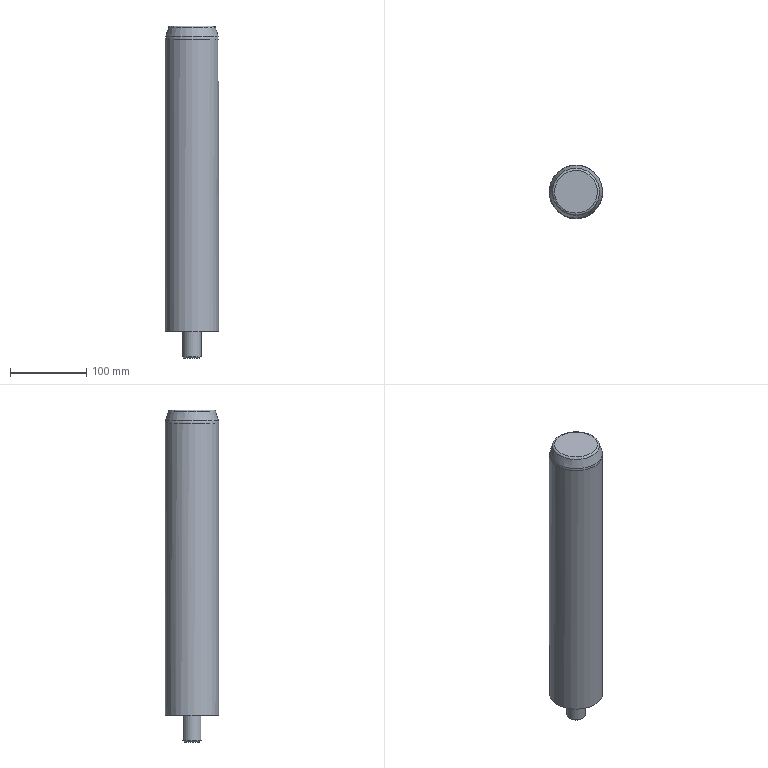Part | STEP file | solid 39 | 1 solid | 9 faces | box 70 x 70 x 435 mm | volume 1546175 mm3 | plane 3 | cylinder 2 | torus 2 | spline 1 | cone 1 | commonest cylinder face diameters 24 x1 70 x1